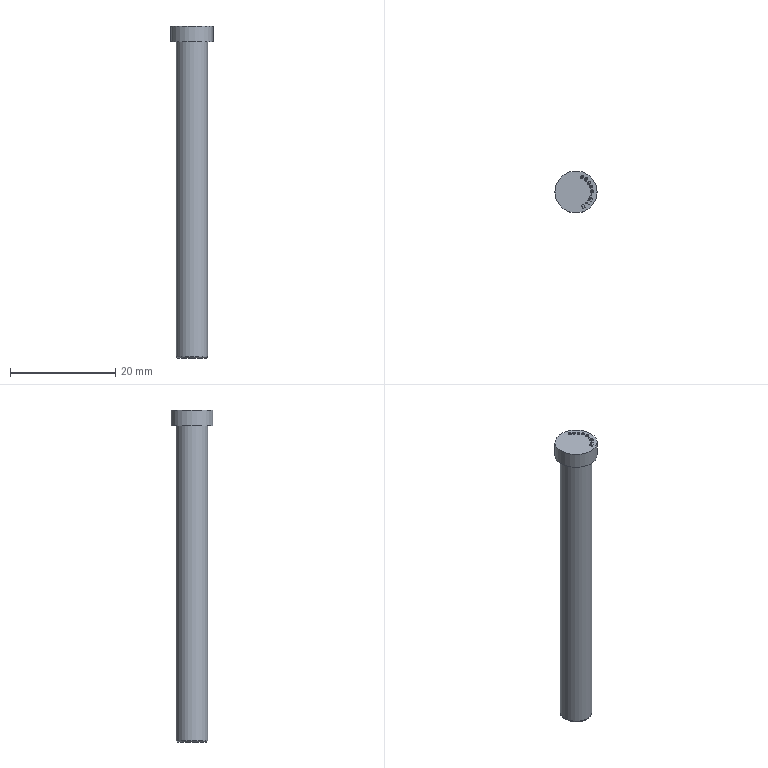Part | STEP file | lll_id2246_x_t | 1 solid | 81 faces | box 8 x 8 x 63 mm | volume 1847 mm3 | plane 48 | other 30 | cylinder 2 | torus 1 | commonest cylinder face diameters 6 x1 8 x1